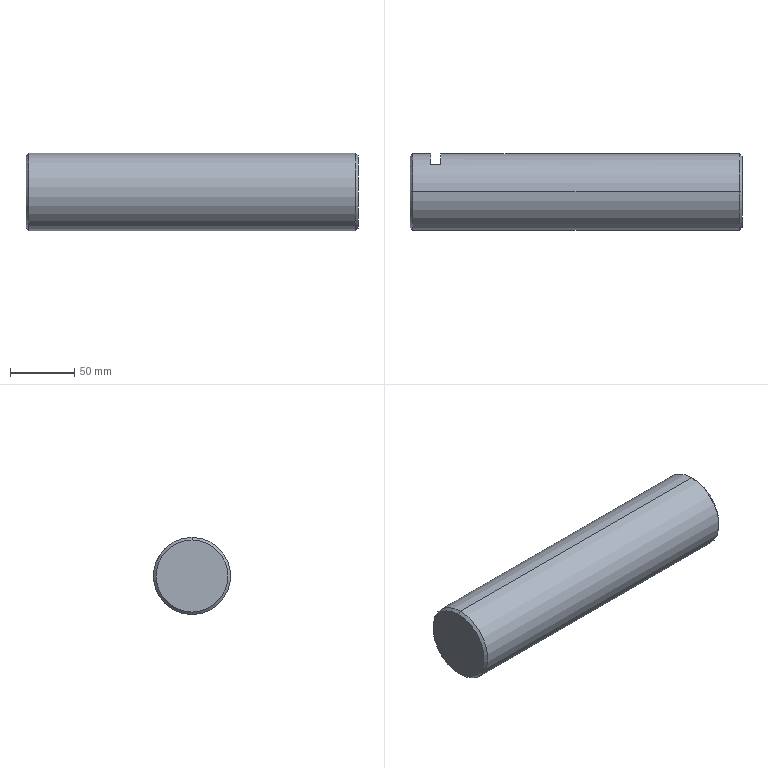Part | STEP file | 04-Driven shaft 2 | 1 solid | 11 faces | box 258 x 60 x 60 mm | volume 726613 mm3 | plane 5 | cone 4 | cylinder 2 | commonest cylinder face diameters 60 x2
STEP:
#1=CARTESIAN_POINT('',(0.,0.,0.));
#2=DIRECTION('',(0.,0.,1.));
#3=DIRECTION('',(1.,0.,0.));
#4=AXIS2_PLACEMENT_3D('',#1,#2,#3);
#5=CARTESIAN_POINT('',(258.,0.,-28.));
#6=VERTEX_POINT('',#5);
#7=CARTESIAN_POINT('',(258.,0.,28.));
#8=VERTEX_POINT('',#7);
#9=CARTESIAN_POINT('',(258.,0.,0.));
#10=DIRECTION('',(1.,0.,0.));
#11=DIRECTION('',(0.,0.,1.));
#12=AXIS2_PLACEMENT_3D('',#9,#10,#11);
#13=CIRCLE('',#12,28.);
#14=CARTESIAN_POINT('',(256.,0.,0.));
#15=DIRECTION('',(-1.,0.,0.));
#16=DIRECTION('',(0.,0.,1.));
#17=AXIS2_PLACEMENT_3D('',#14,#15,#16);
#18=CONICAL_SURFACE('',#17,30.,0.7854);
#19=CARTESIAN_POINT('',(6.283,-2.));
#20=DIRECTION('',(-1.,0.));
#21=VECTOR('',#20,1.);
#22=LINE('',#19,#21);
#23=(GEOMETRIC_REPRESENTATION_CONTEXT(2)PARAMETRIC_REPRESENTATION_CONTEXT()REPRESENTATION_CONTEXT('',''));
#24=DEFINITIONAL_REPRESENTATION('',(#22),#23);
#25=PCURVE('',#18,#24);
#26=CARTESIAN_POINT('',(258.,30.,0.));
#27=DIRECTION('',(-1.,0.,0.));
#28=DIRECTION('',(0.,0.,1.));
#29=AXIS2_PLACEMENT_3D('',#26,#27,#28);
#30=PLANE('',#29);
#31=CARTESIAN_POINT('',(28.,-30.));
#32=CARTESIAN_POINT('',(28.,-78.497));
#33=CARTESIAN_POINT('',(-14.,-54.249));
#34=CARTESIAN_POINT('',(-56.,-30.));
#35=CARTESIAN_POINT('',(-14.,-5.751));
#36=CARTESIAN_POINT('',(28.,18.497));
#37=CARTESIAN_POINT('',(28.,-30.));
#38=(BOUNDED_CURVE()B_SPLINE_CURVE(2,(#31,#32,#33,#34,#35,#36,#37),.UNSPECIFIED.,.T.,.F.)B_SPLINE_CURVE_WITH_KNOTS((1,2,2,2,2,1),(-2.094,0.,2.094,4.189,6.283,8.378),.UNSPECIFIED.)CURVE()GEOMETRIC_REPRESENTATION_ITEM()RATIONAL_B_SPLINE_CURVE((1.,0.5,1.,0.5,1.,0.5,1.))REPRESENTATION_ITEM(''));
#39=(GEOMETRIC_REPRESENTATION_CONTEXT(2)PARAMETRIC_REPRESENTATION_CONTEXT()REPRESENTATION_CONTEXT('',''));
#40=DEFINITIONAL_REPRESENTATION('',(#38),#39);
#41=PCURVE('',#30,#40);
#42=SURFACE_CURVE('',#13,(#25,#41),.PCURVE_S1.);
#43=EDGE_CURVE('',#6,#8,#42,.T.);
#44=ORIENTED_EDGE('',*,*,#43,.F.);
#45=CARTESIAN_POINT('',(256.,0.,-30.));
#46=VERTEX_POINT('',#45);
#47=CARTESIAN_POINT('',(256.,0.,-30.));
#48=DIRECTION('',(-0.7071,0.,-0.7071));
#49=VECTOR('',#48,1.);
#50=LINE('',#47,#49);
#51=CARTESIAN_POINT('',(3.142,0.));
#52=DIRECTION('',(0.,1.));
#53=VECTOR('',#52,1.);
#54=LINE('',#51,#53);
#55=(GEOMETRIC_REPRESENTATION_CONTEXT(2)PARAMETRIC_REPRESENTATION_CONTEXT()REPRESENTATION_CONTEXT('',''));
#56=DEFINITIONAL_REPRESENTATION('',(#54),#55);
#57=PCURVE('',#18,#56);
#58=CARTESIAN_POINT('',(256.,0.,0.));
#59=DIRECTION('',(-1.,0.,0.));
#60=DIRECTION('',(0.,0.,1.));
#61=AXIS2_PLACEMENT_3D('',#58,#59,#60);
#62=CONICAL_SURFACE('',#61,30.,0.7854);
#63=CARTESIAN_POINT('',(3.142,0.));
#64=DIRECTION('',(0.,1.));
#65=VECTOR('',#64,1.);
#66=LINE('',#63,#65);
#67=(GEOMETRIC_REPRESENTATION_CONTEXT(2)PARAMETRIC_REPRESENTATION_CONTEXT()REPRESENTATION_CONTEXT('',''));
#68=DEFINITIONAL_REPRESENTATION('',(#66),#67);
#69=PCURVE('',#62,#68);
#70=SURFACE_CURVE('',#50,(#57,#69),.PCURVE_S1.);
#71=EDGE_CURVE('',#6,#46,#70,.T.);
#72=ORIENTED_EDGE('',*,*,#71,.T.);
#73=CARTESIAN_POINT('',(256.,0.,30.));
#74=VERTEX_POINT('',#73);
#75=CARTESIAN_POINT('',(256.,0.,0.));
#76=DIRECTION('',(-1.,0.,0.));
#77=DIRECTION('',(0.,0.,1.));
#78=AXIS2_PLACEMENT_3D('',#75,#76,#77);
#79=CIRCLE('',#78,30.);
#80=CARTESIAN_POINT('',(0.,0.));
#81=DIRECTION('',(1.,0.));
#82=VECTOR('',#81,1.);
#83=LINE('',#80,#82);
#84=(GEOMETRIC_REPRESENTATION_CONTEXT(2)PARAMETRIC_REPRESENTATION_CONTEXT()REPRESENTATION_CONTEXT('',''));
#85=DEFINITIONAL_REPRESENTATION('',(#83),#84);
#86=PCURVE('',#18,#85);
#87=CARTESIAN_POINT('',(0.,0.,0.));
#88=DIRECTION('',(-1.,0.,0.));
#89=DIRECTION('',(0.,0.,1.));
#90=AXIS2_PLACEMENT_3D('',#87,#88,#89);
#91=CYLINDRICAL_SURFACE('',#90,30.);
#92=CARTESIAN_POINT('',(0.,-256.));
#93=DIRECTION('',(1.,0.));
#94=VECTOR('',#93,1.);
#95=LINE('',#92,#94);
#96=(GEOMETRIC_REPRESENTATION_CONTEXT(2)PARAMETRIC_REPRESENTATION_CONTEXT()REPRESENTATION_CONTEXT('',''));
#97=DEFINITIONAL_REPRESENTATION('',(#95),#96);
#98=PCURVE('',#91,#97);
#99=SURFACE_CURVE('',#79,(#86,#98),.PCURVE_S1.);
#100=EDGE_CURVE('',#74,#46,#99,.T.);
#101=ORIENTED_EDGE('',*,*,#100,.F.);
#102=CARTESIAN_POINT('',(256.,0.,30.));
#103=DIRECTION('',(-0.7071,0.,0.7071));
#104=VECTOR('',#103,1.);
#105=LINE('',#102,#104);
#106=CARTESIAN_POINT('',(0.,0.));
#107=DIRECTION('',(0.,1.));
#108=VECTOR('',#107,1.);
#109=LINE('',#106,#108);
#110=(GEOMETRIC_REPRESENTATION_CONTEXT(2)PARAMETRIC_REPRESENTATION_CONTEXT()REPRESENTATION_CONTEXT('',''));
#111=DEFINITIONAL_REPRESENTATION('',(#109),#110);
#112=PCURVE('',#18,#111);
#113=CARTESIAN_POINT('',(6.283,0.));
#114=DIRECTION('',(0.,1.));
#115=VECTOR('',#114,1.);
#116=LINE('',#113,#115);
#117=(GEOMETRIC_REPRESENTATION_CONTEXT(2)PARAMETRIC_REPRESENTATION_CONTEXT()REPRESENTATION_CONTEXT('',''));
#118=DEFINITIONAL_REPRESENTATION('',(#116),#117);
#119=PCURVE('',#62,#118);
#120=SURFACE_CURVE('',#105,(#112,#119),.PCURVE_S1.);
#121=EDGE_CURVE('',#8,#74,#120,.T.);
#122=ORIENTED_EDGE('',*,*,#121,.F.);
#123=EDGE_LOOP('',(#44,#72,#101,#122));
#124=FACE_BOUND('',#123,.T.);
#125=ADVANCED_FACE('',(#124),#18,.T.);
#126=CARTESIAN_POINT('',(0.,0.,28.));
#127=VERTEX_POINT('',#126);
#128=CARTESIAN_POINT('',(0.,0.,-28.));
#129=VERTEX_POINT('',#128);
#130=CARTESIAN_POINT('',(0.,0.,0.));
#131=DIRECTION('',(-1.,0.,0.));
#132=DIRECTION('',(0.,0.,-1.));
#133=AXIS2_PLACEMENT_3D('',#130,#131,#132);
#134=CIRCLE('',#133,28.);
#135=CARTESIAN_POINT('',(0.,0.,0.));
#136=DIRECTION('',(1.,0.,0.));
#137=DIRECTION('',(0.,0.,-1.));
#138=AXIS2_PLACEMENT_3D('',#135,#136,#137);
#139=CONICAL_SURFACE('',#138,28.,0.7854);
#140=CARTESIAN_POINT('',(6.283,0.));
#141=DIRECTION('',(-1.,0.));
#142=VECTOR('',#141,1.);
#143=LINE('',#140,#142);
#144=(GEOMETRIC_REPRESENTATION_CONTEXT(2)PARAMETRIC_REPRESENTATION_CONTEXT()REPRESENTATION_CONTEXT('',''));
#145=DEFINITIONAL_REPRESENTATION('',(#143),#144);
#146=PCURVE('',#139,#145);
#147=CARTESIAN_POINT('',(0.,0.,0.));
#148=DIRECTION('',(1.,0.,0.));
#149=DIRECTION('',(0.,0.,-1.));
#150=AXIS2_PLACEMENT_3D('',#147,#148,#149);
#151=PLANE('',#150);
#152=CARTESIAN_POINT('',(28.,0.));
#153=CARTESIAN_POINT('',(28.,-48.497));
#154=CARTESIAN_POINT('',(-14.,-24.249));
#155=CARTESIAN_POINT('',(-56.,0.));
#156=CARTESIAN_POINT('',(-14.,24.249));
#157=CARTESIAN_POINT('',(28.,48.497));
#158=CARTESIAN_POINT('',(28.,0.));
#159=(BOUNDED_CURVE()B_SPLINE_CURVE(2,(#152,#153,#154,#155,#156,#157,#158),.UNSPECIFIED.,.T.,.F.)B_SPLINE_CURVE_WITH_KNOTS((1,2,2,2,2,1),(-2.094,0.,2.094,4.189,6.283,8.378),.UNSPECIFIED.)CURVE()GEOMETRIC_REPRESENTATION_ITEM()RATIONAL_B_SPLINE_CURVE((1.,0.5,1.,0.5,1.,0.5,1.))REPRESENTATION_ITEM(''));
#160=(GEOMETRIC_REPRESENTATION_CONTEXT(2)PARAMETRIC_REPRESENTATION_CONTEXT()REPRESENTATION_CONTEXT('',''));
#161=DEFINITIONAL_REPRESENTATION('',(#159),#160);
#162=PCURVE('',#151,#161);
#163=SURFACE_CURVE('',#134,(#146,#162),.PCURVE_S1.);
#164=EDGE_CURVE('',#127,#129,#163,.T.);
#165=ORIENTED_EDGE('',*,*,#164,.F.);
#166=CARTESIAN_POINT('',(2.,0.,30.));
#167=VERTEX_POINT('',#166);
#168=CARTESIAN_POINT('',(0.,0.,28.));
#169=DIRECTION('',(0.7071,0.,0.7071));
#170=VECTOR('',#169,1.);
#171=LINE('',#168,#170);
#172=CARTESIAN_POINT('',(3.142,0.));
#173=DIRECTION('',(0.,1.));
#174=VECTOR('',#173,1.);
#175=LINE('',#172,#174);
#176=(GEOMETRIC_REPRESENTATION_CONTEXT(2)PARAMETRIC_REPRESENTATION_CONTEXT()REPRESENTATION_CONTEXT('',''));
#177=DEFINITIONAL_REPRESENTATION('',(#175),#176);
#178=PCURVE('',#139,#177);
#179=CARTESIAN_POINT('',(0.,0.,0.));
#180=DIRECTION('',(1.,0.,0.));
#181=DIRECTION('',(0.,0.,-1.));
#182=AXIS2_PLACEMENT_3D('',#179,#180,#181);
#183=CONICAL_SURFACE('',#182,28.,0.7854);
#184=CARTESIAN_POINT('',(3.142,0.));
#185=DIRECTION('',(0.,1.));
#186=VECTOR('',#185,1.);
#187=LINE('',#184,#186);
#188=(GEOMETRIC_REPRESENTATION_CONTEXT(2)PARAMETRIC_REPRESENTATION_CONTEXT()REPRESENTATION_CONTEXT('',''));
#189=DEFINITIONAL_REPRESENTATION('',(#187),#188);
#190=PCURVE('',#183,#189);
#191=SURFACE_CURVE('',#171,(#178,#190),.PCURVE_S1.);
#192=EDGE_CURVE('',#127,#167,#191,.T.);
#193=ORIENTED_EDGE('',*,*,#192,.T.);
#194=CARTESIAN_POINT('',(2.,0.,-30.));
#195=VERTEX_POINT('',#194);
#196=CARTESIAN_POINT('',(2.,0.,0.));
#197=DIRECTION('',(1.,0.,0.));
#198=DIRECTION('',(0.,0.,-1.));
#199=AXIS2_PLACEMENT_3D('',#196,#197,#198);
#200=CIRCLE('',#199,30.);
#201=CARTESIAN_POINT('',(0.,2.));
#202=DIRECTION('',(1.,0.));
#203=VECTOR('',#202,1.);
#204=LINE('',#201,#203);
#205=(GEOMETRIC_REPRESENTATION_CONTEXT(2)PARAMETRIC_REPRESENTATION_CONTEXT()REPRESENTATION_CONTEXT('',''));
#206=DEFINITIONAL_REPRESENTATION('',(#204),#205);
#207=PCURVE('',#139,#206);
#208=CARTESIAN_POINT('',(3.142,-2.));
#209=DIRECTION('',(-1.,0.));
#210=VECTOR('',#209,1.);
#211=LINE('',#208,#210);
#212=(GEOMETRIC_REPRESENTATION_CONTEXT(2)PARAMETRIC_REPRESENTATION_CONTEXT()REPRESENTATION_CONTEXT('',''));
#213=DEFINITIONAL_REPRESENTATION('',(#211),#212);
#214=PCURVE('',#91,#213);
#215=SURFACE_CURVE('',#200,(#207,#214),.PCURVE_S1.);
#216=EDGE_CURVE('',#195,#167,#215,.T.);
#217=ORIENTED_EDGE('',*,*,#216,.F.);
#218=CARTESIAN_POINT('',(0.,0.,-28.));
#219=DIRECTION('',(0.7071,0.,-0.7071));
#220=VECTOR('',#219,1.);
#221=LINE('',#218,#220);
#222=CARTESIAN_POINT('',(0.,0.));
#223=DIRECTION('',(0.,1.));
#224=VECTOR('',#223,1.);
#225=LINE('',#222,#224);
#226=(GEOMETRIC_REPRESENTATION_CONTEXT(2)PARAMETRIC_REPRESENTATION_CONTEXT()REPRESENTATION_CONTEXT('',''));
#227=DEFINITIONAL_REPRESENTATION('',(#225),#226);
#228=PCURVE('',#139,#227);
#229=CARTESIAN_POINT('',(6.283,0.));
#230=DIRECTION('',(0.,1.));
#231=VECTOR('',#230,1.);
#232=LINE('',#229,#231);
#233=(GEOMETRIC_REPRESENTATION_CONTEXT(2)PARAMETRIC_REPRESENTATION_CONTEXT()REPRESENTATION_CONTEXT('',''));
#234=DEFINITIONAL_REPRESENTATION('',(#232),#233);
#235=PCURVE('',#183,#234);
#236=SURFACE_CURVE('',#221,(#228,#235),.PCURVE_S1.);
#237=EDGE_CURVE('',#129,#195,#236,.T.);
#238=ORIENTED_EDGE('',*,*,#237,.F.);
#239=EDGE_LOOP('',(#165,#193,#217,#238));
#240=FACE_BOUND('',#239,.T.);
#241=ADVANCED_FACE('',(#240),#139,.T.);
#242=CARTESIAN_POINT('',(24.,21.,-21.424));
#243=VERTEX_POINT('',#242);
#244=CARTESIAN_POINT('',(16.,21.,-21.424));
#245=VERTEX_POINT('',#244);
#246=CARTESIAN_POINT('',(0.,21.,-21.424));
#247=DIRECTION('',(-1.,0.,0.));
#248=VECTOR('',#247,1.);
#249=LINE('',#246,#248);
#250=CARTESIAN_POINT('',(2.366,0.));
#251=DIRECTION('',(0.,1.));
#252=VECTOR('',#251,1.);
#253=LINE('',#250,#252);
#254=(GEOMETRIC_REPRESENTATION_CONTEXT(2)PARAMETRIC_REPRESENTATION_CONTEXT()REPRESENTATION_CONTEXT('',''));
#255=DEFINITIONAL_REPRESENTATION('',(#253),#254);
#256=PCURVE('',#91,#255);
#257=CARTESIAN_POINT('',(0.,21.,0.));
#258=DIRECTION('',(0.,1.,0.));
#259=DIRECTION('',(0.,0.,1.));
#260=AXIS2_PLACEMENT_3D('',#257,#258,#259);
#261=PLANE('',#260);
#262=CARTESIAN_POINT('',(-21.424,0.));
#263=DIRECTION('',(0.,-1.));
#264=VECTOR('',#263,1.);
#265=LINE('',#262,#264);
#266=(GEOMETRIC_REPRESENTATION_CONTEXT(2)PARAMETRIC_REPRESENTATION_CONTEXT()REPRESENTATION_CONTEXT('',''));
#267=DEFINITIONAL_REPRESENTATION('',(#265),#266);
#268=PCURVE('',#261,#267);
#269=SURFACE_CURVE('',#249,(#256,#268),.PCURVE_S1.);
#270=EDGE_CURVE('',#243,#245,#269,.T.);
#271=ORIENTED_EDGE('',*,*,#270,.F.);
#272=CARTESIAN_POINT('',(24.,21.,21.424));
#273=VERTEX_POINT('',#272);
#274=CARTESIAN_POINT('',(24.,0.,0.));
#275=DIRECTION('',(-1.,0.,0.));
#276=DIRECTION('',(0.,0.,1.));
#277=AXIS2_PLACEMENT_3D('',#274,#275,#276);
#278=CIRCLE('',#277,30.);
#279=CARTESIAN_POINT('',(0.,-24.));
#280=DIRECTION('',(1.,0.));
#281=VECTOR('',#280,1.);
#282=LINE('',#279,#281);
#283=(GEOMETRIC_REPRESENTATION_CONTEXT(2)PARAMETRIC_REPRESENTATION_CONTEXT()REPRESENTATION_CONTEXT('',''));
#284=DEFINITIONAL_REPRESENTATION('',(#282),#283);
#285=PCURVE('',#91,#284);
#286=CARTESIAN_POINT('',(24.,31.,-45.622));
#287=DIRECTION('',(-1.,0.,0.));
#288=DIRECTION('',(0.,0.,1.));
#289=AXIS2_PLACEMENT_3D('',#286,#287,#288);
#290=PLANE('',#289);
#291=CARTESIAN_POINT('',(45.622,-31.));
#292=DIRECTION('',(1.,0.));
#293=AXIS2_PLACEMENT_2D('',#291,#292);
#294=CIRCLE('',#293,30.);
#295=(GEOMETRIC_REPRESENTATION_CONTEXT(2)PARAMETRIC_REPRESENTATION_CONTEXT()REPRESENTATION_CONTEXT('',''));
#296=DEFINITIONAL_REPRESENTATION('',(#294),#295);
#297=PCURVE('',#290,#296);
#298=SURFACE_CURVE('',#278,(#285,#297),.PCURVE_S1.);
#299=EDGE_CURVE('',#273,#243,#298,.T.);
#300=ORIENTED_EDGE('',*,*,#299,.F.);
#301=CARTESIAN_POINT('',(16.,21.,21.424));
#302=VERTEX_POINT('',#301);
#303=CARTESIAN_POINT('',(0.,21.,21.424));
#304=DIRECTION('',(1.,0.,0.));
#305=VECTOR('',#304,1.);
#306=LINE('',#303,#305);
#307=CARTESIAN_POINT('',(0.7754,0.));
#308=DIRECTION('',(0.,-1.));
#309=VECTOR('',#308,1.);
#310=LINE('',#307,#309);
#311=(GEOMETRIC_REPRESENTATION_CONTEXT(2)PARAMETRIC_REPRESENTATION_CONTEXT()REPRESENTATION_CONTEXT('',''));
#312=DEFINITIONAL_REPRESENTATION('',(#310),#311);
#313=PCURVE('',#91,#312);
#314=CARTESIAN_POINT('',(21.424,0.));
#315=DIRECTION('',(0.,1.));
#316=VECTOR('',#315,1.);
#317=LINE('',#314,#316);
#318=(GEOMETRIC_REPRESENTATION_CONTEXT(2)PARAMETRIC_REPRESENTATION_CONTEXT()REPRESENTATION_CONTEXT('',''));
#319=DEFINITIONAL_REPRESENTATION('',(#317),#318);
#320=PCURVE('',#261,#319);
#321=SURFACE_CURVE('',#306,(#313,#320),.PCURVE_S1.);
#322=EDGE_CURVE('',#302,#273,#321,.T.);
#323=ORIENTED_EDGE('',*,*,#322,.F.);
#324=CARTESIAN_POINT('',(16.,0.,0.));
#325=DIRECTION('',(1.,0.,0.));
#326=DIRECTION('',(0.,0.,-1.));
#327=AXIS2_PLACEMENT_3D('',#324,#325,#326);
#328=CIRCLE('',#327,30.);
#329=CARTESIAN_POINT('',(3.142,-16.));
#330=DIRECTION('',(-1.,0.));
#331=VECTOR('',#330,1.);
#332=LINE('',#329,#331);
#333=(GEOMETRIC_REPRESENTATION_CONTEXT(2)PARAMETRIC_REPRESENTATION_CONTEXT()REPRESENTATION_CONTEXT('',''));
#334=DEFINITIONAL_REPRESENTATION('',(#332),#333);
#335=PCURVE('',#91,#334);
#336=CARTESIAN_POINT('',(16.,31.,-45.622));
#337=DIRECTION('',(1.,0.,0.));
#338=DIRECTION('',(0.,0.,-1.));
#339=AXIS2_PLACEMENT_3D('',#336,#337,#338);
#340=PLANE('',#339);
#341=CARTESIAN_POINT('',(-45.622,-31.));
#342=DIRECTION('',(1.,0.));
#343=AXIS2_PLACEMENT_2D('',#341,#342);
#344=CIRCLE('',#343,30.);
#345=(GEOMETRIC_REPRESENTATION_CONTEXT(2)PARAMETRIC_REPRESENTATION_CONTEXT()REPRESENTATION_CONTEXT('',''));
#346=DEFINITIONAL_REPRESENTATION('',(#344),#345);
#347=PCURVE('',#340,#346);
#348=SURFACE_CURVE('',#328,(#335,#347),.PCURVE_S1.);
#349=EDGE_CURVE('',#245,#302,#348,.T.);
#350=ORIENTED_EDGE('',*,*,#349,.F.);
#351=EDGE_LOOP('',(#271,#300,#323,#350));
#352=FACE_BOUND('',#351,.T.);
#353=ORIENTED_EDGE('',*,*,#100,.T.);
#354=CARTESIAN_POINT('',(0.,0.,-30.));
#355=DIRECTION('',(-1.,0.,0.));
#356=VECTOR('',#355,1.);
#357=LINE('',#354,#356);
#358=CARTESIAN_POINT('',(3.142,0.));
#359=DIRECTION('',(0.,1.));
#360=VECTOR('',#359,1.);
#361=LINE('',#358,#360);
#362=(GEOMETRIC_REPRESENTATION_CONTEXT(2)PARAMETRIC_REPRESENTATION_CONTEXT()REPRESENTATION_CONTEXT('',''));
#363=DEFINITIONAL_REPRESENTATION('',(#361),#362);
#364=PCURVE('',#91,#363);
#365=CARTESIAN_POINT('',(0.,0.,0.));
#366=DIRECTION('',(-1.,0.,0.));
#367=DIRECTION('',(0.,0.,1.));
#368=AXIS2_PLACEMENT_3D('',#365,#366,#367);
#369=CYLINDRICAL_SURFACE('',#368,30.);
#370=CARTESIAN_POINT('',(3.142,0.));
#371=DIRECTION('',(0.,1.));
#372=VECTOR('',#371,1.);
#373=LINE('',#370,#372);
#374=(GEOMETRIC_REPRESENTATION_CONTEXT(2)PARAMETRIC_REPRESENTATION_CONTEXT()REPRESENTATION_CONTEXT('',''));
#375=DEFINITIONAL_REPRESENTATION('',(#373),#374);
#376=PCURVE('',#369,#375);
#377=SURFACE_CURVE('',#357,(#364,#376),.PCURVE_S1.);
#378=EDGE_CURVE('',#46,#195,#377,.T.);
#379=ORIENTED_EDGE('',*,*,#378,.T.);
#380=ORIENTED_EDGE('',*,*,#216,.T.);
#381=CARTESIAN_POINT('',(0.,0.,30.));
#382=DIRECTION('',(-1.,0.,0.));
#383=VECTOR('',#382,1.);
#384=LINE('',#381,#383);
#385=CARTESIAN_POINT('',(0.,0.));
#386=DIRECTION('',(0.,1.));
#387=VECTOR('',#386,1.);
#388=LINE('',#385,#387);
#389=(GEOMETRIC_REPRESENTATION_CONTEXT(2)PARAMETRIC_REPRESENTATION_CONTEXT()REPRESENTATION_CONTEXT('',''));
#390=DEFINITIONAL_REPRESENTATION('',(#388),#389);
#391=PCURVE('',#91,#390);
#392=CARTESIAN_POINT('',(6.283,0.));
#393=DIRECTION('',(0.,1.));
#394=VECTOR('',#393,1.);
#395=LINE('',#392,#394);
#396=(GEOMETRIC_REPRESENTATION_CONTEXT(2)PARAMETRIC_REPRESENTATION_CONTEXT()REPRESENTATION_CONTEXT('',''));
#397=DEFINITIONAL_REPRESENTATION('',(#395),#396);
#398=PCURVE('',#369,#397);
#399=SURFACE_CURVE('',#384,(#391,#398),.PCURVE_S1.);
#400=EDGE_CURVE('',#74,#167,#399,.T.);
#401=ORIENTED_EDGE('',*,*,#400,.F.);
#402=EDGE_LOOP('',(#353,#379,#380,#401));
#403=FACE_BOUND('',#402,.T.);
#404=ADVANCED_FACE('',(#352,#403),#91,.T.);
#405=ORIENTED_EDGE('',*,*,#378,.F.);
#406=CARTESIAN_POINT('',(256.,0.,0.));
#407=DIRECTION('',(-1.,0.,0.));
#408=DIRECTION('',(0.,0.,1.));
#409=AXIS2_PLACEMENT_3D('',#406,#407,#408);
#410=CIRCLE('',#409,30.);
#411=CARTESIAN_POINT('',(0.,-256.));
#412=DIRECTION('',(1.,0.));
#413=VECTOR('',#412,1.);
#414=LINE('',#411,#413);
#415=(GEOMETRIC_REPRESENTATION_CONTEXT(2)PARAMETRIC_REPRESENTATION_CONTEXT()REPRESENTATION_CONTEXT('',''));
#416=DEFINITIONAL_REPRESENTATION('',(#414),#415);
#417=PCURVE('',#369,#416);
#418=CARTESIAN_POINT('',(0.,0.));
#419=DIRECTION('',(1.,0.));
#420=VECTOR('',#419,1.);
#421=LINE('',#418,#420);
#422=(GEOMETRIC_REPRESENTATION_CONTEXT(2)PARAMETRIC_REPRESENTATION_CONTEXT()REPRESENTATION_CONTEXT('',''));
#423=DEFINITIONAL_REPRESENTATION('',(#421),#422);
#424=PCURVE('',#62,#423);
#425=SURFACE_CURVE('',#410,(#417,#424),.PCURVE_S1.);
#426=EDGE_CURVE('',#46,#74,#425,.T.);
#427=ORIENTED_EDGE('',*,*,#426,.T.);
#428=ORIENTED_EDGE('',*,*,#400,.T.);
#429=CARTESIAN_POINT('',(2.,0.,0.));
#430=DIRECTION('',(1.,0.,0.));
#431=DIRECTION('',(0.,0.,-1.));
#432=AXIS2_PLACEMENT_3D('',#429,#430,#431);
#433=CIRCLE('',#432,30.);
#434=CARTESIAN_POINT('',(9.425,-2.));
#435=DIRECTION('',(-1.,0.));
#436=VECTOR('',#435,1.);
#437=LINE('',#434,#436);
#438=(GEOMETRIC_REPRESENTATION_CONTEXT(2)PARAMETRIC_REPRESENTATION_CONTEXT()REPRESENTATION_CONTEXT('',''));
#439=DEFINITIONAL_REPRESENTATION('',(#437),#438);
#440=PCURVE('',#369,#439);
#441=CARTESIAN_POINT('',(0.,2.));
#442=DIRECTION('',(1.,0.));
#443=VECTOR('',#442,1.);
#444=LINE('',#441,#443);
#445=(GEOMETRIC_REPRESENTATION_CONTEXT(2)PARAMETRIC_REPRESENTATION_CONTEXT()REPRESENTATION_CONTEXT('',''));
#446=DEFINITIONAL_REPRESENTATION('',(#444),#445);
#447=PCURVE('',#183,#446);
#448=SURFACE_CURVE('',#433,(#440,#447),.PCURVE_S1.);
#449=EDGE_CURVE('',#167,#195,#448,.T.);
#450=ORIENTED_EDGE('',*,*,#449,.T.);
#451=EDGE_LOOP('',(#405,#427,#428,#450));
#452=FACE_BOUND('',#451,.T.);
#453=ADVANCED_FACE('',(#452),#369,.T.);
#454=CARTESIAN_POINT('',(0.,0.,0.));
#455=DIRECTION('',(-1.,0.,0.));
#456=DIRECTION('',(0.,0.,-1.));
#457=AXIS2_PLACEMENT_3D('',#454,#455,#456);
#458=CIRCLE('',#457,28.);
#459=CARTESIAN_POINT('',(28.,0.));
#460=CARTESIAN_POINT('',(28.,-48.497));
#461=CARTESIAN_POINT('',(-14.,-24.249));
#462=CARTESIAN_POINT('',(-56.,0.));
#463=CARTESIAN_POINT('',(-14.,24.249));
#464=CARTESIAN_POINT('',(28.,48.497));
#465=CARTESIAN_POINT('',(28.,0.));
#466=(BOUNDED_CURVE()B_SPLINE_CURVE(2,(#459,#460,#461,#462,#463,#464,#465),.UNSPECIFIED.,.T.,.F.)B_SPLINE_CURVE_WITH_KNOTS((1,2,2,2,2,1),(-2.094,0.,2.094,4.189,6.283,8.378),.UNSPECIFIED.)CURVE()GEOMETRIC_REPRESENTATION_ITEM()RATIONAL_B_SPLINE_CURVE((1.,0.5,1.,0.5,1.,0.5,1.))REPRESENTATION_ITEM(''));
#467=(GEOMETRIC_REPRESENTATION_CONTEXT(2)PARAMETRIC_REPRESENTATION_CONTEXT()REPRESENTATION_CONTEXT('',''));
#468=DEFINITIONAL_REPRESENTATION('',(#466),#467);
#469=PCURVE('',#151,#468);
#470=CARTESIAN_POINT('',(6.283,0.));
#471=DIRECTION('',(-1.,0.));
#472=VECTOR('',#471,1.);
#473=LINE('',#470,#472);
#474=(GEOMETRIC_REPRESENTATION_CONTEXT(2)PARAMETRIC_REPRESENTATION_CONTEXT()REPRESENTATION_CONTEXT('',''));
#475=DEFINITIONAL_REPRESENTATION('',(#473),#474);
#476=PCURVE('',#183,#475);
#477=SURFACE_CURVE('',#458,(#469,#476),.PCURVE_S1.);
#478=EDGE_CURVE('',#129,#127,#477,.T.);
#479=ORIENTED_EDGE('',*,*,#478,.T.);
#480=ORIENTED_EDGE('',*,*,#164,.T.);
#481=EDGE_LOOP('',(#479,#480));
#482=FACE_BOUND('',#481,.T.);
#483=ADVANCED_FACE('',(#482),#151,.F.);
#484=CARTESIAN_POINT('',(258.,0.,0.));
#485=DIRECTION('',(1.,0.,0.));
#486=DIRECTION('',(0.,0.,1.));
#487=AXIS2_PLACEMENT_3D('',#484,#485,#486);
#488=CIRCLE('',#487,28.);
#489=CARTESIAN_POINT('',(28.,-30.));
#490=CARTESIAN_POINT('',(28.,-78.497));
#491=CARTESIAN_POINT('',(-14.,-54.249));
#492=CARTESIAN_POINT('',(-56.,-30.));
#493=CARTESIAN_POINT('',(-14.,-5.751));
#494=CARTESIAN_POINT('',(28.,18.497));
#495=CARTESIAN_POINT('',(28.,-30.));
#496=(BOUNDED_CURVE()B_SPLINE_CURVE(2,(#489,#490,#491,#492,#493,#494,#495),.UNSPECIFIED.,.T.,.F.)B_SPLINE_CURVE_WITH_KNOTS((1,2,2,2,2,1),(-2.094,0.,2.094,4.189,6.283,8.378),.UNSPECIFIED.)CURVE()GEOMETRIC_REPRESENTATION_ITEM()RATIONAL_B_SPLINE_CURVE((1.,0.5,1.,0.5,1.,0.5,1.))REPRESENTATION_ITEM(''));
#497=(GEOMETRIC_REPRESENTATION_CONTEXT(2)PARAMETRIC_REPRESENTATION_CONTEXT()REPRESENTATION_CONTEXT('',''));
#498=DEFINITIONAL_REPRESENTATION('',(#496),#497);
#499=PCURVE('',#30,#498);
#500=CARTESIAN_POINT('',(6.283,-2.));
#501=DIRECTION('',(-1.,0.));
#502=VECTOR('',#501,1.);
#503=LINE('',#500,#502);
#504=(GEOMETRIC_REPRESENTATION_CONTEXT(2)PARAMETRIC_REPRESENTATION_CONTEXT()REPRESENTATION_CONTEXT('',''));
#505=DEFINITIONAL_REPRESENTATION('',(#503),#504);
#506=PCURVE('',#62,#505);
#507=SURFACE_CURVE('',#488,(#499,#506),.PCURVE_S1.);
#508=EDGE_CURVE('',#8,#6,#507,.T.);
#509=ORIENTED_EDGE('',*,*,#508,.T.);
#510=ORIENTED_EDGE('',*,*,#43,.T.);
#511=EDGE_LOOP('',(#509,#510));
#512=FACE_BOUND('',#511,.T.);
#513=ADVANCED_FACE('',(#512),#30,.F.);
#514=ORIENTED_EDGE('',*,*,#349,.T.);
#515=CARTESIAN_POINT('',(16.,21.,-45.622));
#516=DIRECTION('',(0.,0.,1.));
#517=VECTOR('',#516,1.);
#518=LINE('',#515,#517);
#519=CARTESIAN_POINT('',(0.,-10.));
#520=DIRECTION('',(-1.,0.));
#521=VECTOR('',#520,1.);
#522=LINE('',#519,#521);
#523=(GEOMETRIC_REPRESENTATION_CONTEXT(2)PARAMETRIC_REPRESENTATION_CONTEXT()REPRESENTATION_CONTEXT('',''));
#524=DEFINITIONAL_REPRESENTATION('',(#522),#523);
#525=PCURVE('',#340,#524);
#526=CARTESIAN_POINT('',(-45.622,16.));
#527=DIRECTION('',(1.,0.));
#528=VECTOR('',#527,1.);
#529=LINE('',#526,#528);
#530=(GEOMETRIC_REPRESENTATION_CONTEXT(2)PARAMETRIC_REPRESENTATION_CONTEXT()REPRESENTATION_CONTEXT('',''));
#531=DEFINITIONAL_REPRESENTATION('',(#529),#530);
#532=PCURVE('',#261,#531);
#533=SURFACE_CURVE('',#518,(#525,#532),.PCURVE_S1.);
#534=EDGE_CURVE('',#245,#302,#533,.T.);
#535=ORIENTED_EDGE('',*,*,#534,.F.);
#536=EDGE_LOOP('',(#514,#535));
#537=FACE_BOUND('',#536,.T.);
#538=ADVANCED_FACE('',(#537),#340,.T.);
#539=ORIENTED_EDGE('',*,*,#299,.T.);
#540=CARTESIAN_POINT('',(24.,21.,-45.622));
#541=DIRECTION('',(0.,0.,-1.));
#542=VECTOR('',#541,1.);
#543=LINE('',#540,#542);
#544=CARTESIAN_POINT('',(0.,-10.));
#545=DIRECTION('',(-1.,0.));
#546=VECTOR('',#545,1.);
#547=LINE('',#544,#546);
#548=(GEOMETRIC_REPRESENTATION_CONTEXT(2)PARAMETRIC_REPRESENTATION_CONTEXT()REPRESENTATION_CONTEXT('',''));
#549=DEFINITIONAL_REPRESENTATION('',(#547),#548);
#550=PCURVE('',#290,#549);
#551=CARTESIAN_POINT('',(-45.622,24.));
#552=DIRECTION('',(-1.,0.));
#553=VECTOR('',#552,1.);
#554=LINE('',#551,#553);
#555=(GEOMETRIC_REPRESENTATION_CONTEXT(2)PARAMETRIC_REPRESENTATION_CONTEXT()REPRESENTATION_CONTEXT('',''));
#556=DEFINITIONAL_REPRESENTATION('',(#554),#555);
#557=PCURVE('',#261,#556);
#558=SURFACE_CURVE('',#543,(#550,#557),.PCURVE_S1.);
#559=EDGE_CURVE('',#273,#243,#558,.T.);
#560=ORIENTED_EDGE('',*,*,#559,.F.);
#561=EDGE_LOOP('',(#539,#560));
#562=FACE_BOUND('',#561,.T.);
#563=ADVANCED_FACE('',(#562),#290,.T.);
#564=ORIENTED_EDGE('',*,*,#270,.T.);
#565=ORIENTED_EDGE('',*,*,#534,.T.);
#566=ORIENTED_EDGE('',*,*,#322,.T.);
#567=ORIENTED_EDGE('',*,*,#559,.T.);
#568=EDGE_LOOP('',(#564,#565,#566,#567));
#569=FACE_BOUND('',#568,.T.);
#570=ADVANCED_FACE('',(#569),#261,.T.);
#571=ORIENTED_EDGE('',*,*,#192,.F.);
#572=ORIENTED_EDGE('',*,*,#478,.F.);
#573=ORIENTED_EDGE('',*,*,#237,.T.);
#574=ORIENTED_EDGE('',*,*,#449,.F.);
#575=EDGE_LOOP('',(#571,#572,#573,#574));
#576=FACE_BOUND('',#575,.T.);
#577=ADVANCED_FACE('',(#576),#183,.T.);
#578=ORIENTED_EDGE('',*,*,#71,.F.);
#579=ORIENTED_EDGE('',*,*,#508,.F.);
#580=ORIENTED_EDGE('',*,*,#121,.T.);
#581=ORIENTED_EDGE('',*,*,#426,.F.);
#582=EDGE_LOOP('',(#578,#579,#580,#581));
#583=FACE_BOUND('',#582,.T.);
#584=ADVANCED_FACE('',(#583),#62,.T.);
#585=CLOSED_SHELL('',(#125,#241,#404,#453,#483,#513,#538,#563,#570,#577,#584));
#586=MANIFOLD_SOLID_BREP('',#585);
#587=(LENGTH_UNIT()NAMED_UNIT(*)SI_UNIT(.MILLI.,.METRE.));
#588=UNCERTAINTY_MEASURE_WITH_UNIT(LENGTH_MEASURE(0.0000001),#587,'','');
#589=(NAMED_UNIT(*)PLANE_ANGLE_UNIT()SI_UNIT($,.RADIAN.));
#590=(NAMED_UNIT(*)SI_UNIT($,.STERADIAN.)SOLID_ANGLE_UNIT());
#591=(GEOMETRIC_REPRESENTATION_CONTEXT(3)GLOBAL_UNCERTAINTY_ASSIGNED_CONTEXT((#588))GLOBAL_UNIT_ASSIGNED_CONTEXT((#587,#589,#590))REPRESENTATION_CONTEXT('',''));
#592=ADVANCED_BREP_SHAPE_REPRESENTATION('',(#4,#586),#591);